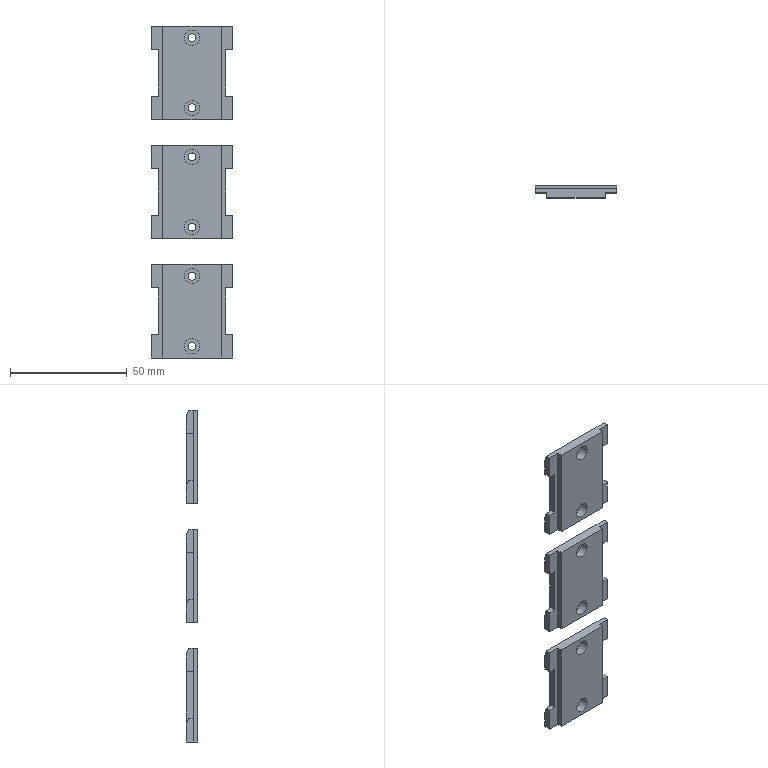Part | 3 solids | 81 faces | box 35 x 5 x 142 mm | volume 16587 mm3 | plane 69 | cylinder 12 | commonest cylinder face diameters 3.4 x6 6.5 x6